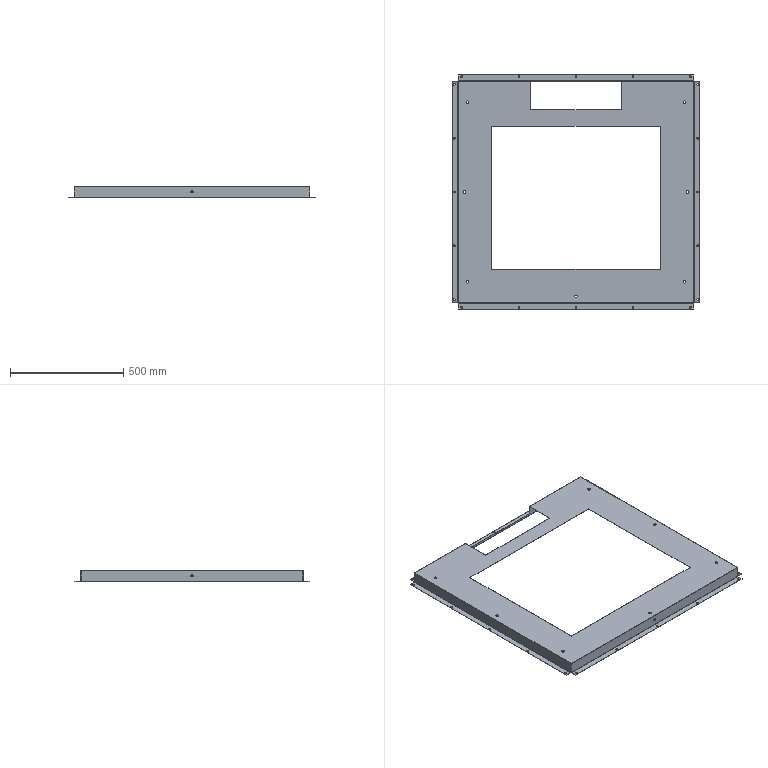Part | SolidWorks | features ICE 7, EdgeFlange 2, FlatPattern 1, SMBaseFlange 1, SheetMetal 1 | 1 solid | 194 faces | box 1095 x 1035 x 50 mm | volume 787160 mm3 | plane 98 | cylinder 88 | spline 8 | commonest cylinder face diameters 7 x50 11 x14 0.4 x9 2.4 x9 10 x6